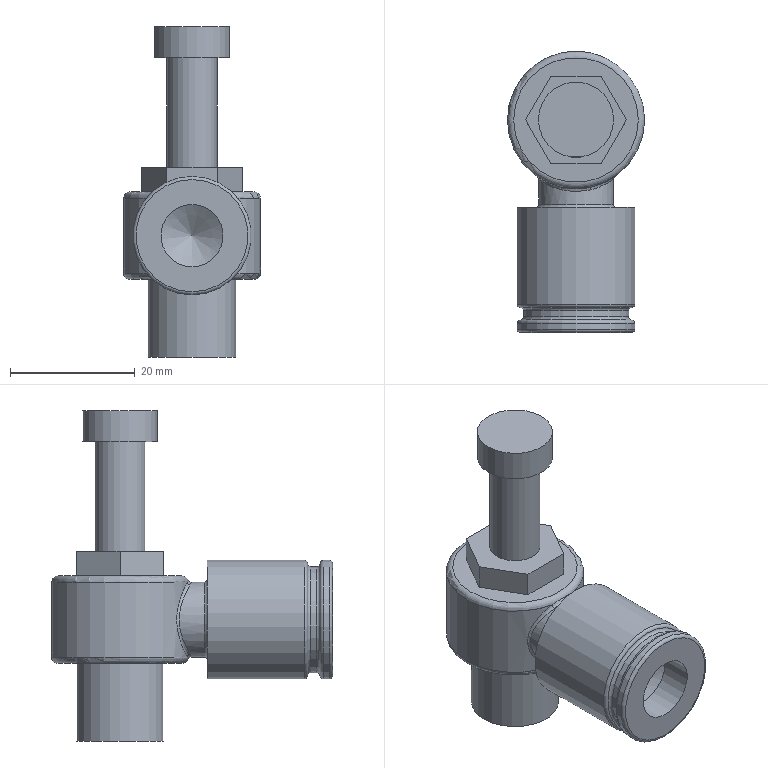Part | STEP file | Tube feed_id730_x_t | 1 solid | 36 faces | box 22 x 45.08 x 53 mm | volume 14856 mm3 | plane 14 | cylinder 9 | torus 8 | spline 4 | cone 1 | commonest cylinder face diameters 19 x2 8.06 x1 10 x1 12 x1 12.06 x1 14 x1